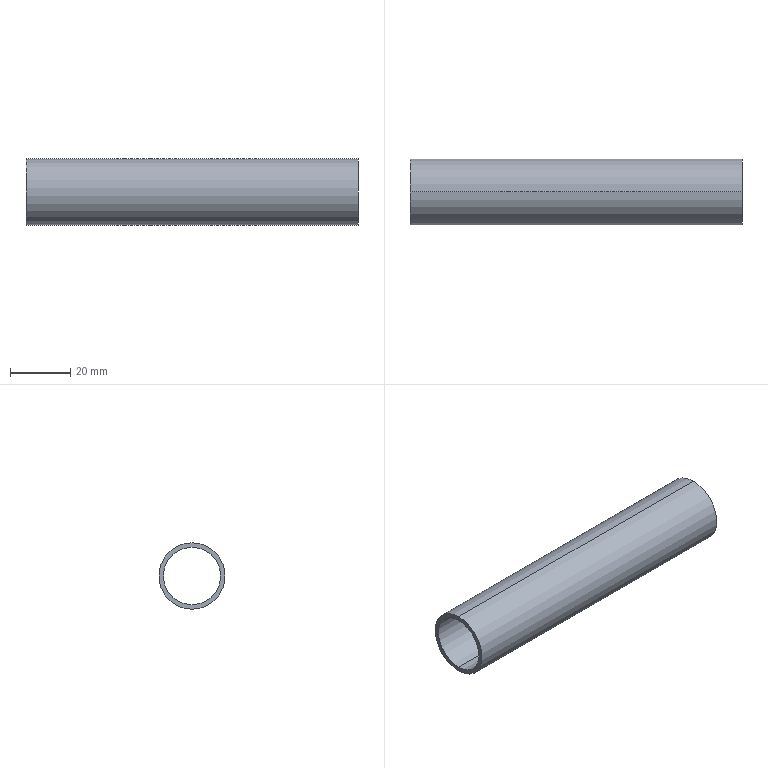Part | STEP file | copper tube 13_default_machined_ | 1 solid | 6 faces | box 110 x 22 x 22 mm | volume 10626 mm3 | cylinder 4 | plane 2 | commonest cylinder face diameters 19 x2 22 x2
STEP:
#1=CARTESIAN_POINT('',(0.,0.,0.));
#2=DIRECTION('',(0.,0.,1.));
#3=DIRECTION('',(1.,0.,0.));
#4=AXIS2_PLACEMENT_3D('',#1,#2,#3);
#5=CARTESIAN_POINT('',(110.,0.,11.));
#6=VERTEX_POINT('',#5);
#7=CARTESIAN_POINT('',(110.,0.,-11.));
#8=VERTEX_POINT('',#7);
#9=CARTESIAN_POINT('',(110.,0.,0.));
#10=DIRECTION('',(-1.,0.,0.));
#11=DIRECTION('',(0.,0.,1.));
#12=AXIS2_PLACEMENT_3D('',#9,#10,#11);
#13=CIRCLE('',#12,11.);
#14=CARTESIAN_POINT('',(110.,0.,0.));
#15=DIRECTION('',(-1.,0.,0.));
#16=DIRECTION('',(0.,0.,1.));
#17=AXIS2_PLACEMENT_3D('',#14,#15,#16);
#18=CYLINDRICAL_SURFACE('',#17,11.);
#19=CARTESIAN_POINT('',(0.,0.));
#20=DIRECTION('',(1.,0.));
#21=VECTOR('',#20,1.);
#22=LINE('',#19,#21);
#23=(GEOMETRIC_REPRESENTATION_CONTEXT(2)PARAMETRIC_REPRESENTATION_CONTEXT()REPRESENTATION_CONTEXT('',''));
#24=DEFINITIONAL_REPRESENTATION('',(#22),#23);
#25=PCURVE('',#18,#24);
#26=CARTESIAN_POINT('',(110.,0.,0.));
#27=DIRECTION('',(1.,0.,0.));
#28=DIRECTION('',(0.,0.,-1.));
#29=AXIS2_PLACEMENT_3D('',#26,#27,#28);
#30=PLANE('',#29);
#31=CARTESIAN_POINT('',(-11.,0.));
#32=CARTESIAN_POINT('',(-11.,19.053));
#33=CARTESIAN_POINT('',(5.5,9.526));
#34=CARTESIAN_POINT('',(22.,0.));
#35=CARTESIAN_POINT('',(5.5,-9.526));
#36=CARTESIAN_POINT('',(-11.,-19.053));
#37=CARTESIAN_POINT('',(-11.,0.));
#38=(BOUNDED_CURVE()B_SPLINE_CURVE(2,(#31,#32,#33,#34,#35,#36,#37),.UNSPECIFIED.,.T.,.F.)B_SPLINE_CURVE_WITH_KNOTS((1,2,2,2,2,1),(-2.094,0.,2.094,4.189,6.283,8.378),.UNSPECIFIED.)CURVE()GEOMETRIC_REPRESENTATION_ITEM()RATIONAL_B_SPLINE_CURVE((1.,0.5,1.,0.5,1.,0.5,1.))REPRESENTATION_ITEM(''));
#39=(GEOMETRIC_REPRESENTATION_CONTEXT(2)PARAMETRIC_REPRESENTATION_CONTEXT()REPRESENTATION_CONTEXT('',''));
#40=DEFINITIONAL_REPRESENTATION('',(#38),#39);
#41=PCURVE('',#30,#40);
#42=SURFACE_CURVE('',#13,(#25,#41),.PCURVE_S1.);
#43=EDGE_CURVE('',#6,#8,#42,.T.);
#44=ORIENTED_EDGE('',*,*,#43,.T.);
#45=CARTESIAN_POINT('',(0.,0.,-11.));
#46=VERTEX_POINT('',#45);
#47=CARTESIAN_POINT('',(110.,0.,-11.));
#48=DIRECTION('',(-1.,0.,0.));
#49=VECTOR('',#48,1.);
#50=LINE('',#47,#49);
#51=CARTESIAN_POINT('',(3.142,0.));
#52=DIRECTION('',(0.,1.));
#53=VECTOR('',#52,1.);
#54=LINE('',#51,#53);
#55=(GEOMETRIC_REPRESENTATION_CONTEXT(2)PARAMETRIC_REPRESENTATION_CONTEXT()REPRESENTATION_CONTEXT('',''));
#56=DEFINITIONAL_REPRESENTATION('',(#54),#55);
#57=PCURVE('',#18,#56);
#58=CARTESIAN_POINT('',(110.,0.,0.));
#59=DIRECTION('',(-1.,0.,0.));
#60=DIRECTION('',(0.,0.,1.));
#61=AXIS2_PLACEMENT_3D('',#58,#59,#60);
#62=CYLINDRICAL_SURFACE('',#61,11.);
#63=CARTESIAN_POINT('',(3.142,0.));
#64=DIRECTION('',(0.,1.));
#65=VECTOR('',#64,1.);
#66=LINE('',#63,#65);
#67=(GEOMETRIC_REPRESENTATION_CONTEXT(2)PARAMETRIC_REPRESENTATION_CONTEXT()REPRESENTATION_CONTEXT('',''));
#68=DEFINITIONAL_REPRESENTATION('',(#66),#67);
#69=PCURVE('',#62,#68);
#70=SURFACE_CURVE('',#50,(#57,#69),.PCURVE_S1.);
#71=EDGE_CURVE('',#8,#46,#70,.T.);
#72=ORIENTED_EDGE('',*,*,#71,.T.);
#73=CARTESIAN_POINT('',(0.,0.,11.));
#74=VERTEX_POINT('',#73);
#75=CARTESIAN_POINT('',(0.,0.,0.));
#76=DIRECTION('',(1.,0.,0.));
#77=DIRECTION('',(0.,0.,1.));
#78=AXIS2_PLACEMENT_3D('',#75,#76,#77);
#79=CIRCLE('',#78,11.);
#80=CARTESIAN_POINT('',(6.283,110.));
#81=DIRECTION('',(-1.,0.));
#82=VECTOR('',#81,1.);
#83=LINE('',#80,#82);
#84=(GEOMETRIC_REPRESENTATION_CONTEXT(2)PARAMETRIC_REPRESENTATION_CONTEXT()REPRESENTATION_CONTEXT('',''));
#85=DEFINITIONAL_REPRESENTATION('',(#83),#84);
#86=PCURVE('',#18,#85);
#87=CARTESIAN_POINT('',(0.,0.,0.));
#88=DIRECTION('',(1.,0.,0.));
#89=DIRECTION('',(0.,0.,-1.));
#90=AXIS2_PLACEMENT_3D('',#87,#88,#89);
#91=PLANE('',#90);
#92=CARTESIAN_POINT('',(0.,0.));
#93=DIRECTION('',(-1.,0.));
#94=AXIS2_PLACEMENT_2D('',#92,#93);
#95=CIRCLE('',#94,11.);
#96=(GEOMETRIC_REPRESENTATION_CONTEXT(2)PARAMETRIC_REPRESENTATION_CONTEXT()REPRESENTATION_CONTEXT('',''));
#97=DEFINITIONAL_REPRESENTATION('',(#95),#96);
#98=PCURVE('',#91,#97);
#99=SURFACE_CURVE('',#79,(#86,#98),.PCURVE_S1.);
#100=EDGE_CURVE('',#46,#74,#99,.T.);
#101=ORIENTED_EDGE('',*,*,#100,.T.);
#102=CARTESIAN_POINT('',(110.,0.,11.));
#103=DIRECTION('',(-1.,0.,0.));
#104=VECTOR('',#103,1.);
#105=LINE('',#102,#104);
#106=CARTESIAN_POINT('',(0.,0.));
#107=DIRECTION('',(0.,1.));
#108=VECTOR('',#107,1.);
#109=LINE('',#106,#108);
#110=(GEOMETRIC_REPRESENTATION_CONTEXT(2)PARAMETRIC_REPRESENTATION_CONTEXT()REPRESENTATION_CONTEXT('',''));
#111=DEFINITIONAL_REPRESENTATION('',(#109),#110);
#112=PCURVE('',#18,#111);
#113=CARTESIAN_POINT('',(6.283,0.));
#114=DIRECTION('',(0.,1.));
#115=VECTOR('',#114,1.);
#116=LINE('',#113,#115);
#117=(GEOMETRIC_REPRESENTATION_CONTEXT(2)PARAMETRIC_REPRESENTATION_CONTEXT()REPRESENTATION_CONTEXT('',''));
#118=DEFINITIONAL_REPRESENTATION('',(#116),#117);
#119=PCURVE('',#62,#118);
#120=SURFACE_CURVE('',#105,(#112,#119),.PCURVE_S1.);
#121=EDGE_CURVE('',#6,#74,#120,.T.);
#122=ORIENTED_EDGE('',*,*,#121,.F.);
#123=EDGE_LOOP('',(#44,#72,#101,#122));
#124=FACE_BOUND('',#123,.T.);
#125=ADVANCED_FACE('',(#124),#18,.T.);
#126=CARTESIAN_POINT('',(110.,0.,9.5));
#127=VERTEX_POINT('',#126);
#128=CARTESIAN_POINT('',(0.,0.,9.5));
#129=VERTEX_POINT('',#128);
#130=CARTESIAN_POINT('',(110.,0.,9.5));
#131=DIRECTION('',(-1.,0.,0.));
#132=VECTOR('',#131,1.);
#133=LINE('',#130,#132);
#134=CARTESIAN_POINT('',(110.,0.,0.));
#135=DIRECTION('',(-1.,0.,0.));
#136=DIRECTION('',(0.,0.,1.));
#137=AXIS2_PLACEMENT_3D('',#134,#135,#136);
#138=CYLINDRICAL_SURFACE('',#137,9.5);
#139=CARTESIAN_POINT('',(6.283,0.));
#140=DIRECTION('',(0.,1.));
#141=VECTOR('',#140,1.);
#142=LINE('',#139,#141);
#143=(GEOMETRIC_REPRESENTATION_CONTEXT(2)PARAMETRIC_REPRESENTATION_CONTEXT()REPRESENTATION_CONTEXT('',''));
#144=DEFINITIONAL_REPRESENTATION('',(#142),#143);
#145=PCURVE('',#138,#144);
#146=CARTESIAN_POINT('',(110.,0.,0.));
#147=DIRECTION('',(-1.,0.,0.));
#148=DIRECTION('',(0.,0.,1.));
#149=AXIS2_PLACEMENT_3D('',#146,#147,#148);
#150=CYLINDRICAL_SURFACE('',#149,9.5);
#151=CARTESIAN_POINT('',(0.,0.));
#152=DIRECTION('',(0.,1.));
#153=VECTOR('',#152,1.);
#154=LINE('',#151,#153);
#155=(GEOMETRIC_REPRESENTATION_CONTEXT(2)PARAMETRIC_REPRESENTATION_CONTEXT()REPRESENTATION_CONTEXT('',''));
#156=DEFINITIONAL_REPRESENTATION('',(#154),#155);
#157=PCURVE('',#150,#156);
#158=SURFACE_CURVE('',#133,(#145,#157),.PCURVE_S1.);
#159=EDGE_CURVE('',#127,#129,#158,.T.);
#160=ORIENTED_EDGE('',*,*,#159,.T.);
#161=CARTESIAN_POINT('',(0.,0.,-9.5));
#162=VERTEX_POINT('',#161);
#163=CARTESIAN_POINT('',(0.,0.,0.));
#164=DIRECTION('',(-1.,0.,0.));
#165=DIRECTION('',(0.,0.,1.));
#166=AXIS2_PLACEMENT_3D('',#163,#164,#165);
#167=CIRCLE('',#166,9.5);
#168=CARTESIAN_POINT('',(0.,110.));
#169=DIRECTION('',(1.,0.));
#170=VECTOR('',#169,1.);
#171=LINE('',#168,#170);
#172=(GEOMETRIC_REPRESENTATION_CONTEXT(2)PARAMETRIC_REPRESENTATION_CONTEXT()REPRESENTATION_CONTEXT('',''));
#173=DEFINITIONAL_REPRESENTATION('',(#171),#172);
#174=PCURVE('',#138,#173);
#175=CARTESIAN_POINT('',(-9.5,0.));
#176=CARTESIAN_POINT('',(-9.5,16.454));
#177=CARTESIAN_POINT('',(4.75,8.227));
#178=CARTESIAN_POINT('',(19.,0.));
#179=CARTESIAN_POINT('',(4.75,-8.227));
#180=CARTESIAN_POINT('',(-9.5,-16.454));
#181=CARTESIAN_POINT('',(-9.5,0.));
#182=(BOUNDED_CURVE()B_SPLINE_CURVE(2,(#175,#176,#177,#178,#179,#180,#181),.UNSPECIFIED.,.T.,.F.)B_SPLINE_CURVE_WITH_KNOTS((1,2,2,2,2,1),(-2.094,0.,2.094,4.189,6.283,8.378),.UNSPECIFIED.)CURVE()GEOMETRIC_REPRESENTATION_ITEM()RATIONAL_B_SPLINE_CURVE((1.,0.5,1.,0.5,1.,0.5,1.))REPRESENTATION_ITEM(''));
#183=(GEOMETRIC_REPRESENTATION_CONTEXT(2)PARAMETRIC_REPRESENTATION_CONTEXT()REPRESENTATION_CONTEXT('',''));
#184=DEFINITIONAL_REPRESENTATION('',(#182),#183);
#185=PCURVE('',#91,#184);
#186=SURFACE_CURVE('',#167,(#174,#185),.PCURVE_S1.);
#187=EDGE_CURVE('',#162,#129,#186,.T.);
#188=ORIENTED_EDGE('',*,*,#187,.F.);
#189=CARTESIAN_POINT('',(110.,0.,-9.5));
#190=VERTEX_POINT('',#189);
#191=CARTESIAN_POINT('',(110.,0.,-9.5));
#192=DIRECTION('',(-1.,0.,0.));
#193=VECTOR('',#192,1.);
#194=LINE('',#191,#193);
#195=CARTESIAN_POINT('',(3.142,0.));
#196=DIRECTION('',(0.,1.));
#197=VECTOR('',#196,1.);
#198=LINE('',#195,#197);
#199=(GEOMETRIC_REPRESENTATION_CONTEXT(2)PARAMETRIC_REPRESENTATION_CONTEXT()REPRESENTATION_CONTEXT('',''));
#200=DEFINITIONAL_REPRESENTATION('',(#198),#199);
#201=PCURVE('',#138,#200);
#202=CARTESIAN_POINT('',(3.142,0.));
#203=DIRECTION('',(0.,1.));
#204=VECTOR('',#203,1.);
#205=LINE('',#202,#204);
#206=(GEOMETRIC_REPRESENTATION_CONTEXT(2)PARAMETRIC_REPRESENTATION_CONTEXT()REPRESENTATION_CONTEXT('',''));
#207=DEFINITIONAL_REPRESENTATION('',(#205),#206);
#208=PCURVE('',#150,#207);
#209=SURFACE_CURVE('',#194,(#201,#208),.PCURVE_S1.);
#210=EDGE_CURVE('',#190,#162,#209,.T.);
#211=ORIENTED_EDGE('',*,*,#210,.F.);
#212=CARTESIAN_POINT('',(110.,0.,0.));
#213=DIRECTION('',(-1.,0.,0.));
#214=DIRECTION('',(0.,0.,1.));
#215=AXIS2_PLACEMENT_3D('',#212,#213,#214);
#216=CIRCLE('',#215,9.5);
#217=CARTESIAN_POINT('',(0.,0.));
#218=DIRECTION('',(1.,0.));
#219=VECTOR('',#218,1.);
#220=LINE('',#217,#219);
#221=(GEOMETRIC_REPRESENTATION_CONTEXT(2)PARAMETRIC_REPRESENTATION_CONTEXT()REPRESENTATION_CONTEXT('',''));
#222=DEFINITIONAL_REPRESENTATION('',(#220),#221);
#223=PCURVE('',#138,#222);
#224=CARTESIAN_POINT('',(-9.5,0.));
#225=CARTESIAN_POINT('',(-9.5,16.454));
#226=CARTESIAN_POINT('',(4.75,8.227));
#227=CARTESIAN_POINT('',(19.,0.));
#228=CARTESIAN_POINT('',(4.75,-8.227));
#229=CARTESIAN_POINT('',(-9.5,-16.454));
#230=CARTESIAN_POINT('',(-9.5,0.));
#231=(BOUNDED_CURVE()B_SPLINE_CURVE(2,(#224,#225,#226,#227,#228,#229,#230),.UNSPECIFIED.,.T.,.F.)B_SPLINE_CURVE_WITH_KNOTS((1,2,2,2,2,1),(-2.094,0.,2.094,4.189,6.283,8.378),.UNSPECIFIED.)CURVE()GEOMETRIC_REPRESENTATION_ITEM()RATIONAL_B_SPLINE_CURVE((1.,0.5,1.,0.5,1.,0.5,1.))REPRESENTATION_ITEM(''));
#232=(GEOMETRIC_REPRESENTATION_CONTEXT(2)PARAMETRIC_REPRESENTATION_CONTEXT()REPRESENTATION_CONTEXT('',''));
#233=DEFINITIONAL_REPRESENTATION('',(#231),#232);
#234=PCURVE('',#30,#233);
#235=SURFACE_CURVE('',#216,(#223,#234),.PCURVE_S1.);
#236=EDGE_CURVE('',#190,#127,#235,.T.);
#237=ORIENTED_EDGE('',*,*,#236,.T.);
#238=EDGE_LOOP('',(#160,#188,#211,#237));
#239=FACE_BOUND('',#238,.F.);
#240=ADVANCED_FACE('',(#239),#138,.F.);
#241=ORIENTED_EDGE('',*,*,#71,.F.);
#242=CARTESIAN_POINT('',(110.,0.,0.));
#243=DIRECTION('',(-1.,0.,0.));
#244=DIRECTION('',(0.,0.,1.));
#245=AXIS2_PLACEMENT_3D('',#242,#243,#244);
#246=CIRCLE('',#245,11.);
#247=CARTESIAN_POINT('',(0.,0.));
#248=DIRECTION('',(1.,0.));
#249=VECTOR('',#248,1.);
#250=LINE('',#247,#249);
#251=(GEOMETRIC_REPRESENTATION_CONTEXT(2)PARAMETRIC_REPRESENTATION_CONTEXT()REPRESENTATION_CONTEXT('',''));
#252=DEFINITIONAL_REPRESENTATION('',(#250),#251);
#253=PCURVE('',#62,#252);
#254=CARTESIAN_POINT('',(-11.,0.));
#255=CARTESIAN_POINT('',(-11.,19.053));
#256=CARTESIAN_POINT('',(5.5,9.526));
#257=CARTESIAN_POINT('',(22.,0.));
#258=CARTESIAN_POINT('',(5.5,-9.526));
#259=CARTESIAN_POINT('',(-11.,-19.053));
#260=CARTESIAN_POINT('',(-11.,0.));
#261=(BOUNDED_CURVE()B_SPLINE_CURVE(2,(#254,#255,#256,#257,#258,#259,#260),.UNSPECIFIED.,.T.,.F.)B_SPLINE_CURVE_WITH_KNOTS((1,2,2,2,2,1),(-2.094,0.,2.094,4.189,6.283,8.378),.UNSPECIFIED.)CURVE()GEOMETRIC_REPRESENTATION_ITEM()RATIONAL_B_SPLINE_CURVE((1.,0.5,1.,0.5,1.,0.5,1.))REPRESENTATION_ITEM(''));
#262=(GEOMETRIC_REPRESENTATION_CONTEXT(2)PARAMETRIC_REPRESENTATION_CONTEXT()REPRESENTATION_CONTEXT('',''));
#263=DEFINITIONAL_REPRESENTATION('',(#261),#262);
#264=PCURVE('',#30,#263);
#265=SURFACE_CURVE('',#246,(#253,#264),.PCURVE_S1.);
#266=EDGE_CURVE('',#8,#6,#265,.T.);
#267=ORIENTED_EDGE('',*,*,#266,.T.);
#268=ORIENTED_EDGE('',*,*,#121,.T.);
#269=CARTESIAN_POINT('',(0.,0.,0.));
#270=DIRECTION('',(1.,0.,0.));
#271=DIRECTION('',(0.,0.,1.));
#272=AXIS2_PLACEMENT_3D('',#269,#270,#271);
#273=CIRCLE('',#272,11.);
#274=CARTESIAN_POINT('',(6.283,110.));
#275=DIRECTION('',(-1.,0.));
#276=VECTOR('',#275,1.);
#277=LINE('',#274,#276);
#278=(GEOMETRIC_REPRESENTATION_CONTEXT(2)PARAMETRIC_REPRESENTATION_CONTEXT()REPRESENTATION_CONTEXT('',''));
#279=DEFINITIONAL_REPRESENTATION('',(#277),#278);
#280=PCURVE('',#62,#279);
#281=CARTESIAN_POINT('',(0.,0.));
#282=DIRECTION('',(-1.,0.));
#283=AXIS2_PLACEMENT_2D('',#281,#282);
#284=CIRCLE('',#283,11.);
#285=(GEOMETRIC_REPRESENTATION_CONTEXT(2)PARAMETRIC_REPRESENTATION_CONTEXT()REPRESENTATION_CONTEXT('',''));
#286=DEFINITIONAL_REPRESENTATION('',(#284),#285);
#287=PCURVE('',#91,#286);
#288=SURFACE_CURVE('',#273,(#280,#287),.PCURVE_S1.);
#289=EDGE_CURVE('',#74,#46,#288,.T.);
#290=ORIENTED_EDGE('',*,*,#289,.T.);
#291=EDGE_LOOP('',(#241,#267,#268,#290));
#292=FACE_BOUND('',#291,.T.);
#293=ADVANCED_FACE('',(#292),#62,.T.);
#294=ORIENTED_EDGE('',*,*,#289,.F.);
#295=ORIENTED_EDGE('',*,*,#100,.F.);
#296=EDGE_LOOP('',(#294,#295));
#297=FACE_BOUND('',#296,.T.);
#298=CARTESIAN_POINT('',(0.,0.,0.));
#299=DIRECTION('',(-1.,0.,0.));
#300=DIRECTION('',(0.,0.,1.));
#301=AXIS2_PLACEMENT_3D('',#298,#299,#300);
#302=CIRCLE('',#301,9.5);
#303=CARTESIAN_POINT('',(-9.5,0.));
#304=CARTESIAN_POINT('',(-9.5,16.454));
#305=CARTESIAN_POINT('',(4.75,8.227));
#306=CARTESIAN_POINT('',(19.,0.));
#307=CARTESIAN_POINT('',(4.75,-8.227));
#308=CARTESIAN_POINT('',(-9.5,-16.454));
#309=CARTESIAN_POINT('',(-9.5,0.));
#310=(BOUNDED_CURVE()B_SPLINE_CURVE(2,(#303,#304,#305,#306,#307,#308,#309),.UNSPECIFIED.,.T.,.F.)B_SPLINE_CURVE_WITH_KNOTS((1,2,2,2,2,1),(-2.094,0.,2.094,4.189,6.283,8.378),.UNSPECIFIED.)CURVE()GEOMETRIC_REPRESENTATION_ITEM()RATIONAL_B_SPLINE_CURVE((1.,0.5,1.,0.5,1.,0.5,1.))REPRESENTATION_ITEM(''));
#311=(GEOMETRIC_REPRESENTATION_CONTEXT(2)PARAMETRIC_REPRESENTATION_CONTEXT()REPRESENTATION_CONTEXT('',''));
#312=DEFINITIONAL_REPRESENTATION('',(#310),#311);
#313=PCURVE('',#91,#312);
#314=CARTESIAN_POINT('',(0.,110.));
#315=DIRECTION('',(1.,0.));
#316=VECTOR('',#315,1.);
#317=LINE('',#314,#316);
#318=(GEOMETRIC_REPRESENTATION_CONTEXT(2)PARAMETRIC_REPRESENTATION_CONTEXT()REPRESENTATION_CONTEXT('',''));
#319=DEFINITIONAL_REPRESENTATION('',(#317),#318);
#320=PCURVE('',#150,#319);
#321=SURFACE_CURVE('',#302,(#313,#320),.PCURVE_S1.);
#322=EDGE_CURVE('',#129,#162,#321,.T.);
#323=ORIENTED_EDGE('',*,*,#322,.F.);
#324=ORIENTED_EDGE('',*,*,#187,.F.);
#325=EDGE_LOOP('',(#323,#324));
#326=FACE_BOUND('',#325,.T.);
#327=ADVANCED_FACE('',(#297,#326),#91,.F.);
#328=ORIENTED_EDGE('',*,*,#43,.F.);
#329=ORIENTED_EDGE('',*,*,#266,.F.);
#330=EDGE_LOOP('',(#328,#329));
#331=FACE_BOUND('',#330,.T.);
#332=CARTESIAN_POINT('',(110.,0.,0.));
#333=DIRECTION('',(-1.,0.,0.));
#334=DIRECTION('',(0.,0.,1.));
#335=AXIS2_PLACEMENT_3D('',#332,#333,#334);
#336=CIRCLE('',#335,9.5);
#337=CARTESIAN_POINT('',(-9.5,0.));
#338=CARTESIAN_POINT('',(-9.5,16.454));
#339=CARTESIAN_POINT('',(4.75,8.227));
#340=CARTESIAN_POINT('',(19.,0.));
#341=CARTESIAN_POINT('',(4.75,-8.227));
#342=CARTESIAN_POINT('',(-9.5,-16.454));
#343=CARTESIAN_POINT('',(-9.5,0.));
#344=(BOUNDED_CURVE()B_SPLINE_CURVE(2,(#337,#338,#339,#340,#341,#342,#343),.UNSPECIFIED.,.T.,.F.)B_SPLINE_CURVE_WITH_KNOTS((1,2,2,2,2,1),(-2.094,0.,2.094,4.189,6.283,8.378),.UNSPECIFIED.)CURVE()GEOMETRIC_REPRESENTATION_ITEM()RATIONAL_B_SPLINE_CURVE((1.,0.5,1.,0.5,1.,0.5,1.))REPRESENTATION_ITEM(''));
#345=(GEOMETRIC_REPRESENTATION_CONTEXT(2)PARAMETRIC_REPRESENTATION_CONTEXT()REPRESENTATION_CONTEXT('',''));
#346=DEFINITIONAL_REPRESENTATION('',(#344),#345);
#347=PCURVE('',#30,#346);
#348=CARTESIAN_POINT('',(0.,0.));
#349=DIRECTION('',(1.,0.));
#350=VECTOR('',#349,1.);
#351=LINE('',#348,#350);
#352=(GEOMETRIC_REPRESENTATION_CONTEXT(2)PARAMETRIC_REPRESENTATION_CONTEXT()REPRESENTATION_CONTEXT('',''));
#353=DEFINITIONAL_REPRESENTATION('',(#351),#352);
#354=PCURVE('',#150,#353);
#355=SURFACE_CURVE('',#336,(#347,#354),.PCURVE_S1.);
#356=EDGE_CURVE('',#127,#190,#355,.T.);
#357=ORIENTED_EDGE('',*,*,#356,.T.);
#358=ORIENTED_EDGE('',*,*,#236,.T.);
#359=EDGE_LOOP('',(#357,#358));
#360=FACE_BOUND('',#359,.T.);
#361=ADVANCED_FACE('',(#331,#360),#30,.T.);
#362=ORIENTED_EDGE('',*,*,#322,.F.);
#363=ORIENTED_EDGE('',*,*,#159,.F.);
#364=ORIENTED_EDGE('',*,*,#356,.T.);
#365=ORIENTED_EDGE('',*,*,#210,.T.);
#366=EDGE_LOOP('',(#362,#363,#364,#365));
#367=FACE_BOUND('',#366,.F.);
#368=ADVANCED_FACE('',(#367),#150,.F.);
#369=CLOSED_SHELL('',(#125,#240,#293,#327,#361,#368));
#370=MANIFOLD_SOLID_BREP('',#369);
#371=(LENGTH_UNIT()NAMED_UNIT(*)SI_UNIT(.MILLI.,.METRE.));
#372=UNCERTAINTY_MEASURE_WITH_UNIT(LENGTH_MEASURE(0.0000001),#371,'','');
#373=(NAMED_UNIT(*)PLANE_ANGLE_UNIT()SI_UNIT($,.RADIAN.));
#374=(NAMED_UNIT(*)SI_UNIT($,.STERADIAN.)SOLID_ANGLE_UNIT());
#375=(GEOMETRIC_REPRESENTATION_CONTEXT(3)GLOBAL_UNCERTAINTY_ASSIGNED_CONTEXT((#372))GLOBAL_UNIT_ASSIGNED_CONTEXT((#371,#373,#374))REPRESENTATION_CONTEXT('',''));
#376=ADVANCED_BREP_SHAPE_REPRESENTATION('',(#4,#370),#375);